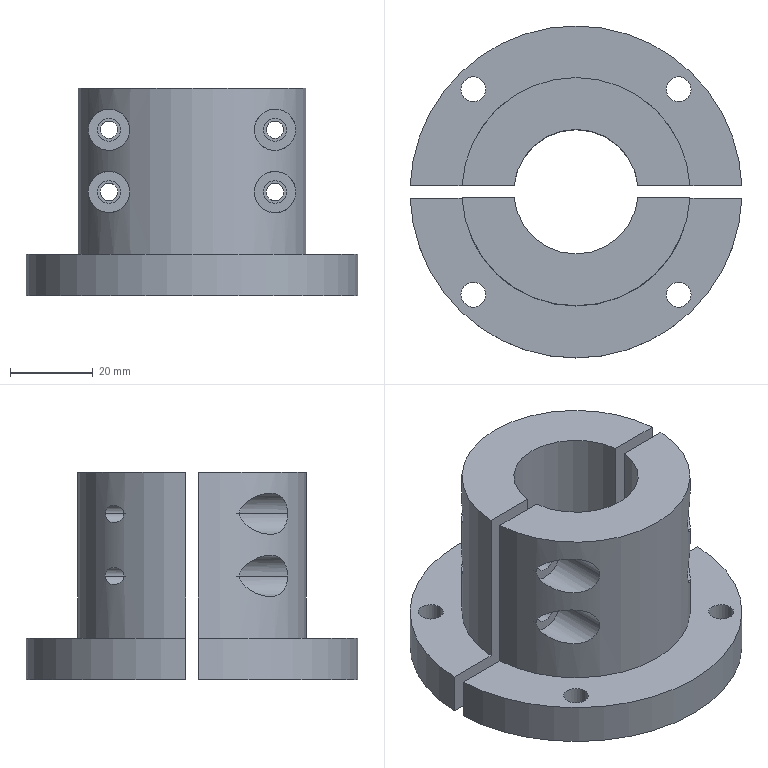NC program | NX | posted with a generic post | part box 79.944 x 80 x 50 mm
Whole program:
N10 G17 G21 G94 G90
(HOLE_MILLING , TOOL : D6)
N12 T12 M6
N14 G54
N16 G17 G0 G90 X-20. Y0. B0. C0. S9500 M3
N18 G43 Z68.5 H12
N20 Z22.549
N22 G94 G3 X-21. Y1. R1. F1500.
N24 X-22. Y0. R1.
N26 X-22. Y0. Z22.049 I2. J0.
N28 X-22. Y0. Z21.549 I2. J0.
N30 X-22. Y0. Z21.049 I2. J0.
N32 X-22. Y0. Z20.549 I2. J0.
N34 X-22. Y0. Z20.049 I2. J0.
N36 X-22. Y0. Z19.549 I2. J0.
N38 X-22. Y0. Z19.049 I2. J0.
N40 X-22. Y0. Z18.549 I2. J0.
N42 X-22. Y0. Z18.049 I2. J0.
N44 X-22. Y0. Z17.549 I2. J0.
N46 X-22. Y0. Z17.049 I2. J0.
N48 X-22. Y0. Z16.549 I2. J0.
N50 X-22. Y0. Z16.049 I2. J0.
N52 X-22. Y0. Z15.549 I2. J0.
N54 X-22. Y0. Z15.049 I2. J0.
N56 X-22. Y0. Z14.549 I2. J0.
N58 X-22. Y0. Z14.049 I2. J0.
N60 X-22. Y0. Z13.549 I2. J0.
N62 X-22. Y0. Z13.049 I2. J0.
N64 X-22. Y0. Z12.549 I2. J0.
N66 X-22. Y0. Z12.049 I2. J0.
N68 X-22. Y0. Z11.549 I2. J0.
N70 X-22. Y0. Z11.049 I2. J0.
N72 X-22. Y0. Z10.549 I2. J0.
N74 X-22. Y0. Z10.049 I2. J0.
N76 X-22. Y0. Z9.549 I2. J0.
N78 X-22. Y0. Z9.049 I2. J0.
N80 X-22. Y0. Z8.549 I2. J0.
N82 X-22. Y0. Z8.049 I2. J0.
N84 X-21.635 Y-1.152 Z8. R2.
N86 X-18.848 Y-1.635 R2.
N88 X-21.635 Y-1.152 R-2.
N90 X-20.241 Y-1.393 R1.
N92 X-20. Y0. R1.
N94 G0 Z68.5
N96 Y-15.
N98 Z22.549
N100 G3 X-21. Y-14. R1.
N102 X-22. Y-15. R1.
N104 X-22. Y-15. Z22.049 I2. J0.
N106 X-22. Y-15. Z21.549 I2. J0.
N108 X-22. Y-15. Z21.049 I2. J0.
N110 X-22. Y-15. Z20.549 I2. J0.
N112 X-22. Y-15. Z20.049 I2. J0.
N114 X-22. Y-15. Z19.549 I2. J0.
N116 X-22. Y-15. Z19.049 I2. J0.
N118 X-22. Y-15. Z18.549 I2. J0.
N120 X-22. Y-15. Z18.049 I2. J0.
N122 X-22. Y-15. Z17.549 I2. J0.
N124 X-22. Y-15. Z17.049 I2. J0.
N126 X-22. Y-15. Z16.549 I2. J0.
N128 X-22. Y-15. Z16.049 I2. J0.
N130 X-22. Y-15. Z15.549 I2. J0.
N132 X-22. Y-15. Z15.049 I2. J0.
N134 X-22. Y-15. Z14.549 I2. J0.
N136 X-22. Y-15. Z14.049 I2. J0.
N138 X-22. Y-15. Z13.549 I2. J0.
N140 X-22. Y-15. Z13.049 I2. J0.
N142 X-22. Y-15. Z12.549 I2. J0.
N144 X-22. Y-15. Z12.049 I2. J0.
N146 X-22. Y-15. Z11.549 I2. J0.
N148 X-22. Y-15. Z11.049 I2. J0.
N150 X-22. Y-15. Z10.549 I2. J0.
N152 X-22. Y-15. Z10.049 I2. J0.
N154 X-22. Y-15. Z9.549 I2. J0.
N156 X-22. Y-15. Z9.049 I2. J0.
N158 X-22. Y-15. Z8.549 I2. J0.
N160 X-22. Y-15. Z8.049 I2. J0.
N162 X-21.635 Y-16.152 Z8. R2.
N164 X-18.848 Y-16.635 R2.
N166 X-21.635 Y-16.152 R-2.
N168 X-20.241 Y-16.393 R1.
N170 X-20. Y-15. R1.
N172 G0 Z68.5
N174 X20.
N176 Z22.549
N178 G3 X19. Y-14. R1.
N180 X18. Y-15. R1.
N182 X18. Y-15. Z22.049 I2. J0.
N184 X18. Y-15. Z21.549 I2. J0.
N186 X18. Y-15. Z21.049 I2. J0.
N188 X18. Y-15. Z20.549 I2. J0.
N190 X18. Y-15. Z20.049 I2. J0.
N192 X18. Y-15. Z19.549 I2. J0.
N194 X18. Y-15. Z19.049 I2. J0.
N196 X18. Y-15. Z18.549 I2. J0.
N198 X18. Y-15. Z18.049 I2. J0.
N200 X18. Y-15. Z17.549 I2. J0.
N202 X18. Y-15. Z17.049 I2. J0.
N204 X18. Y-15. Z16.549 I2. J0.
N206 X18. Y-15. Z16.049 I2. J0.
N208 X18. Y-15. Z15.549 I2. J0.
N210 X18. Y-15. Z15.049 I2. J0.
N212 X18. Y-15. Z14.549 I2. J0.
N214 X18. Y-15. Z14.049 I2. J0.
N216 X18. Y-15. Z13.549 I2. J0.
N218 X18. Y-15. Z13.049 I2. J0.
N220 X18. Y-15. Z12.549 I2. J0.
N222 X18. Y-15. Z12.049 I2. J0.
N224 X18. Y-15. Z11.549 I2. J0.
N226 X18. Y-15. Z11.049 I2. J0.
N228 X18. Y-15. Z10.549 I2. J0.
N230 X18. Y-15. Z10.049 I2. J0.
N232 X18. Y-15. Z9.549 I2. J0.
N234 X18. Y-15. Z9.049 I2. J0.
N236 X18. Y-15. Z8.549 I2. J0.
N238 X18. Y-15. Z8.049 I2. J0.
N240 X18.365 Y-16.152 Z8. R2.
N242 X21.152 Y-16.635 R2.
N244 X18.365 Y-16.152 R-2.
N246 X19.759 Y-16.393 R1.
N248 X20. Y-15. R1.
N250 G0 Z68.5
N252 Y0.
N254 Z22.549
N256 G3 X19. Y1. R1.
N258 X18. Y0. R1.
N260 X18. Y0. Z22.049 I2. J0.
N262 X18. Y0. Z21.549 I2. J0.
N264 X18. Y0. Z21.049 I2. J0.
N266 X18. Y0. Z20.549 I2. J0.
N268 X18. Y0. Z20.049 I2. J0.
N270 X18. Y0. Z19.549 I2. J0.
N272 X18. Y0. Z19.049 I2. J0.
N274 X18. Y0. Z18.549 I2. J0.
N276 X18. Y0. Z18.049 I2. J0.
N278 X18. Y0. Z17.549 I2. J0.
N280 X18. Y0. Z17.049 I2. J0.
N282 X18. Y0. Z16.549 I2. J0.
N284 X18. Y0. Z16.049 I2. J0.
N286 X18. Y0. Z15.549 I2. J0.
N288 X18. Y0. Z15.049 I2. J0.
N290 X18. Y0. Z14.549 I2. J0.
N292 X18. Y0. Z14.049 I2. J0.
N294 X18. Y0. Z13.549 I2. J0.
N296 X18. Y0. Z13.049 I2. J0.
N298 X18. Y0. Z12.549 I2. J0.
N300 X18. Y0. Z12.049 I2. J0.
N302 X18. Y0. Z11.549 I2. J0.
N304 X18. Y0. Z11.049 I2. J0.
N306 X18. Y0. Z10.549 I2. J0.
N308 X18. Y0. Z10.049 I2. J0.
N310 X18. Y0. Z9.549 I2. J0.
N312 X18. Y0. Z9.049 I2. J0.
N314 X18. Y0. Z8.549 I2. J0.
N316 X18. Y0. Z8.049 I2. J0.
N318 X18.365 Y-1.152 Z8. R2.
N320 X21.152 Y-1.635 R2.
N322 X18.365 Y-1.152 R-2.
N324 X19.759 Y-1.393 R1.
N326 X20. Y0. R1.
N328 G0 Z68.5
N330 M5
(DRILLING_COPY_1_COPY , TOOL : D6A45)
N332 T01 M6
N334 G54
N336 G17 G0 G90 X-20. Y0. B0. C0. S5000 M3
N338 G43 Z68.5 H1
N340 G94 G81 G98 Z7. F350. R11.
N342 Y-15.
N344 X20.
N346 Y0.
N348 G80
N350 G0 X20. Y0. Z68.5
N352 M5
(DRILLING_COPY_1_COPY_COPY_COPY , TOOL : 5.5ZT)
N354 T09 M6
N356 G54
N358 G17 G0 G90 X-20. Y0. B0. C0. S2000 M3
N360 G43 Z68.5 H9
N362 G94 G83 G98 Z-3.152 F200. Q2. R11.
N364 Y-15.
N366 X20.
N368 Y0.
N370 G80
N372 G0 X20. Y0. Z68.5
N374 M5
N376 M2